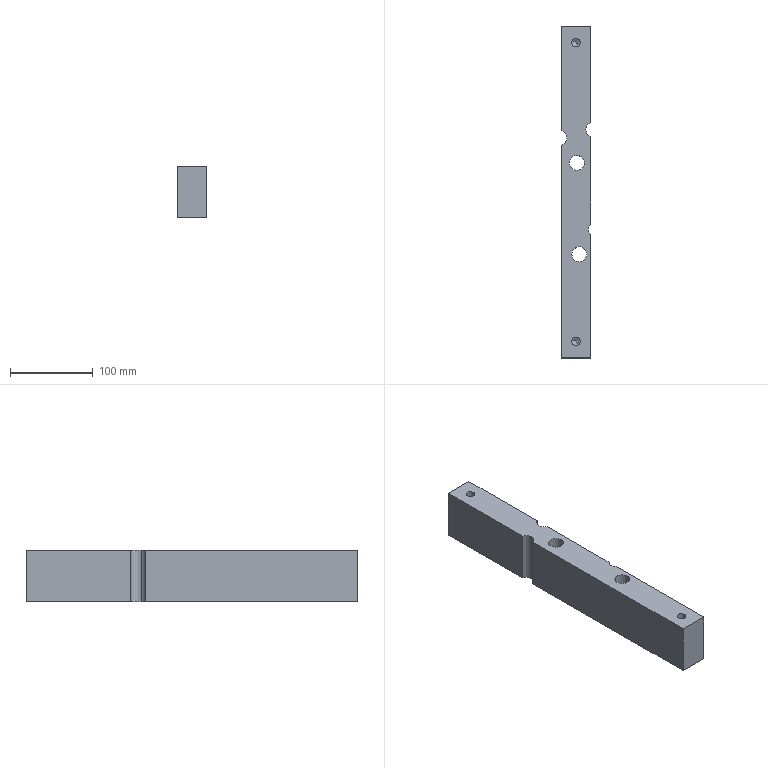Part | CATIA | 1 solid | 39 faces | box 35 x 400 x 61.7 mm | volume 807204 mm3 | cylinder 20 | cone 10 | plane 9 | commonest cylinder face diameters 10.2 x10 18 x10
STEP:
#1=CARTESIAN_POINT('',(-17.5,-200.,-275.));
#2=VERTEX_POINT('',#1);
#3=CARTESIAN_POINT('',(17.5,-200.,-275.));
#4=VERTEX_POINT('',#3);
#5=CARTESIAN_POINT('',(0.,-200.,-275.));
#6=DIRECTION('',(-1.,0.,0.));
#7=VECTOR('',#6,1.);
#8=LINE('',#5,#7);
#9=EDGE_CURVE('',#2,#4,#8,.F.);
#10=ORIENTED_EDGE('',*,*,#9,.T.);
#11=CARTESIAN_POINT('',(17.5,-200.,-213.3));
#12=VERTEX_POINT('',#11);
#13=CARTESIAN_POINT('',(17.5,-200.,-244.15));
#14=DIRECTION('',(0.,0.,-1.));
#15=VECTOR('',#14,1.);
#16=LINE('',#13,#15);
#17=EDGE_CURVE('',#12,#4,#16,.T.);
#18=ORIENTED_EDGE('',*,*,#17,.F.);
#19=CARTESIAN_POINT('',(-17.5,-200.,-213.3));
#20=VERTEX_POINT('',#19);
#21=CARTESIAN_POINT('',(0.,-200.,-213.3));
#22=DIRECTION('',(-1.,0.,0.));
#23=VECTOR('',#22,1.);
#24=LINE('',#21,#23);
#25=EDGE_CURVE('',#20,#12,#24,.F.);
#26=ORIENTED_EDGE('',*,*,#25,.F.);
#27=CARTESIAN_POINT('',(-17.5,-200.,-244.15));
#28=DIRECTION('',(0.,0.,-1.));
#29=VECTOR('',#28,1.);
#30=LINE('',#27,#29);
#31=EDGE_CURVE('',#20,#2,#30,.T.);
#32=ORIENTED_EDGE('',*,*,#31,.T.);
#33=EDGE_LOOP('',(#10,#18,#26,#32));
#34=FACE_OUTER_BOUND('',#33,.T.);
#35=CARTESIAN_POINT('',(17.5,-200.,0.));
#36=DIRECTION('',(0.,-1.,0.));
#37=DIRECTION('',(-1.,0.,0.));
#38=AXIS2_PLACEMENT_3D('',#35,#36,#37);
#39=PLANE('',#38);
#40=ADVANCED_FACE('',(#34),#39,.T.);
#41=CARTESIAN_POINT('',(17.5,200.,-275.));
#42=VERTEX_POINT('',#41);
#43=CARTESIAN_POINT('',(-17.5,200.,-275.));
#44=VERTEX_POINT('',#43);
#45=CARTESIAN_POINT('',(0.,200.,-275.));
#46=DIRECTION('',(1.,0.,0.));
#47=VECTOR('',#46,1.);
#48=LINE('',#45,#47);
#49=EDGE_CURVE('',#42,#44,#48,.F.);
#50=ORIENTED_EDGE('',*,*,#49,.T.);
#51=CARTESIAN_POINT('',(-17.5,200.,-213.3));
#52=VERTEX_POINT('',#51);
#53=CARTESIAN_POINT('',(-17.5,200.,-244.15));
#54=DIRECTION('',(0.,0.,-1.));
#55=VECTOR('',#54,1.);
#56=LINE('',#53,#55);
#57=EDGE_CURVE('',#52,#44,#56,.T.);
#58=ORIENTED_EDGE('',*,*,#57,.F.);
#59=CARTESIAN_POINT('',(17.5,200.,-213.3));
#60=VERTEX_POINT('',#59);
#61=CARTESIAN_POINT('',(0.,200.,-213.3));
#62=DIRECTION('',(1.,0.,0.));
#63=VECTOR('',#62,1.);
#64=LINE('',#61,#63);
#65=EDGE_CURVE('',#60,#52,#64,.F.);
#66=ORIENTED_EDGE('',*,*,#65,.F.);
#67=CARTESIAN_POINT('',(17.5,200.,-244.15));
#68=DIRECTION('',(0.,0.,-1.));
#69=VECTOR('',#68,1.);
#70=LINE('',#67,#69);
#71=EDGE_CURVE('',#60,#42,#70,.T.);
#72=ORIENTED_EDGE('',*,*,#71,.T.);
#73=EDGE_LOOP('',(#50,#58,#66,#72));
#74=FACE_OUTER_BOUND('',#73,.T.);
#75=CARTESIAN_POINT('',(-17.5,200.,0.));
#76=DIRECTION('',(0.,1.,0.));
#77=DIRECTION('',(1.,0.,0.));
#78=AXIS2_PLACEMENT_3D('',#75,#76,#77);
#79=PLANE('',#78);
#80=ADVANCED_FACE('',(#74),#79,.T.);
#81=CARTESIAN_POINT('',(17.5,-38.775,-213.3));
#82=VERTEX_POINT('',#81);
#83=CARTESIAN_POINT('',(17.5,-38.775,-275.));
#84=VERTEX_POINT('',#83);
#85=CARTESIAN_POINT('',(17.5,-38.775,-244.15));
#86=DIRECTION('',(0.,0.,-1.));
#87=VECTOR('',#86,1.);
#88=LINE('',#85,#87);
#89=EDGE_CURVE('',#82,#84,#88,.T.);
#90=ORIENTED_EDGE('',*,*,#89,.T.);
#91=CARTESIAN_POINT('',(17.5,66.708,-275.));
#92=VERTEX_POINT('',#91);
#93=CARTESIAN_POINT('',(17.5,13.967,-275.));
#94=DIRECTION('',(0.,1.,0.));
#95=VECTOR('',#94,1.);
#96=LINE('',#93,#95);
#97=EDGE_CURVE('',#84,#92,#96,.T.);
#98=ORIENTED_EDGE('',*,*,#97,.T.);
#99=CARTESIAN_POINT('',(17.5,66.708,-213.3));
#100=VERTEX_POINT('',#99);
#101=CARTESIAN_POINT('',(17.5,66.708,-244.15));
#102=DIRECTION('',(0.,0.,-1.));
#103=VECTOR('',#102,1.);
#104=LINE('',#101,#103);
#105=EDGE_CURVE('',#100,#92,#104,.T.);
#106=ORIENTED_EDGE('',*,*,#105,.F.);
#107=CARTESIAN_POINT('',(17.5,13.967,-213.3));
#108=DIRECTION('',(0.,1.,0.));
#109=VECTOR('',#108,1.);
#110=LINE('',#107,#109);
#111=EDGE_CURVE('',#82,#100,#110,.T.);
#112=ORIENTED_EDGE('',*,*,#111,.F.);
#113=EDGE_LOOP('',(#90,#98,#106,#112));
#114=FACE_OUTER_BOUND('',#113,.T.);
#115=CARTESIAN_POINT('',(17.5,-200.,0.));
#116=DIRECTION('',(-1.,0.,0.));
#117=DIRECTION('',(0.,1.,0.));
#118=AXIS2_PLACEMENT_3D('',#115,#116,#117);
#119=PLANE('',#118);
#120=ADVANCED_FACE('',(#114),#119,.F.);
#121=CARTESIAN_POINT('',(17.5,-51.225,-213.3));
#122=VERTEX_POINT('',#121);
#123=CARTESIAN_POINT('',(17.5,-51.225,-275.));
#124=VERTEX_POINT('',#123);
#125=CARTESIAN_POINT('',(17.5,-51.225,-244.15));
#126=DIRECTION('',(0.,0.,-1.));
#127=VECTOR('',#126,1.);
#128=LINE('',#125,#127);
#129=EDGE_CURVE('',#122,#124,#128,.T.);
#130=ORIENTED_EDGE('',*,*,#129,.F.);
#131=CARTESIAN_POINT('',(17.5,-125.612,-213.3));
#132=DIRECTION('',(0.,1.,0.));
#133=VECTOR('',#132,1.);
#134=LINE('',#131,#133);
#135=EDGE_CURVE('',#12,#122,#134,.T.);
#136=ORIENTED_EDGE('',*,*,#135,.F.);
#137=ORIENTED_EDGE('',*,*,#17,.T.);
#138=CARTESIAN_POINT('',(17.5,-125.612,-275.));
#139=DIRECTION('',(0.,1.,0.));
#140=VECTOR('',#139,1.);
#141=LINE('',#138,#140);
#142=EDGE_CURVE('',#4,#124,#141,.T.);
#143=ORIENTED_EDGE('',*,*,#142,.T.);
#144=EDGE_LOOP('',(#130,#136,#137,#143));
#145=FACE_OUTER_BOUND('',#144,.T.);
#146=ADVANCED_FACE('',(#145),#119,.F.);
#147=CARTESIAN_POINT('',(17.5,83.292,-213.3));
#148=VERTEX_POINT('',#147);
#149=CARTESIAN_POINT('',(17.5,83.292,-275.));
#150=VERTEX_POINT('',#149);
#151=CARTESIAN_POINT('',(17.5,83.292,-244.15));
#152=DIRECTION('',(0.,0.,-1.));
#153=VECTOR('',#152,1.);
#154=LINE('',#151,#153);
#155=EDGE_CURVE('',#148,#150,#154,.T.);
#156=ORIENTED_EDGE('',*,*,#155,.T.);
#157=CARTESIAN_POINT('',(17.5,141.646,-275.));
#158=DIRECTION('',(0.,1.,0.));
#159=VECTOR('',#158,1.);
#160=LINE('',#157,#159);
#161=EDGE_CURVE('',#150,#42,#160,.T.);
#162=ORIENTED_EDGE('',*,*,#161,.T.);
#163=ORIENTED_EDGE('',*,*,#71,.F.);
#164=CARTESIAN_POINT('',(17.5,141.646,-213.3));
#165=DIRECTION('',(0.,1.,0.));
#166=VECTOR('',#165,1.);
#167=LINE('',#164,#166);
#168=EDGE_CURVE('',#148,#60,#167,.T.);
#169=ORIENTED_EDGE('',*,*,#168,.F.);
#170=EDGE_LOOP('',(#156,#162,#163,#169));
#171=FACE_OUTER_BOUND('',#170,.T.);
#172=ADVANCED_FACE('',(#171),#119,.F.);
#173=CARTESIAN_POINT('',(-17.5,56.354,-213.3));
#174=VERTEX_POINT('',#173);
#175=CARTESIAN_POINT('',(-17.5,56.354,-275.));
#176=VERTEX_POINT('',#175);
#177=CARTESIAN_POINT('',(-17.5,56.354,-244.15));
#178=DIRECTION('',(0.,0.,-1.));
#179=VECTOR('',#178,1.);
#180=LINE('',#177,#179);
#181=EDGE_CURVE('',#174,#176,#180,.T.);
#182=ORIENTED_EDGE('',*,*,#181,.T.);
#183=CARTESIAN_POINT('',(-17.5,-71.823,-275.));
#184=DIRECTION('',(0.,-1.,0.));
#185=VECTOR('',#184,1.);
#186=LINE('',#183,#185);
#187=EDGE_CURVE('',#176,#2,#186,.T.);
#188=ORIENTED_EDGE('',*,*,#187,.T.);
#189=ORIENTED_EDGE('',*,*,#31,.F.);
#190=CARTESIAN_POINT('',(-17.5,-71.823,-213.3));
#191=DIRECTION('',(0.,-1.,0.));
#192=VECTOR('',#191,1.);
#193=LINE('',#190,#192);
#194=EDGE_CURVE('',#174,#20,#193,.T.);
#195=ORIENTED_EDGE('',*,*,#194,.F.);
#196=EDGE_LOOP('',(#182,#188,#189,#195));
#197=FACE_OUTER_BOUND('',#196,.T.);
#198=CARTESIAN_POINT('',(-17.5,200.,0.));
#199=DIRECTION('',(1.,0.,0.));
#200=DIRECTION('',(0.,-1.,0.));
#201=AXIS2_PLACEMENT_3D('',#198,#199,#200);
#202=PLANE('',#201);
#203=ADVANCED_FACE('',(#197),#202,.F.);
#204=CARTESIAN_POINT('',(-17.5,73.646,-213.3));
#205=VERTEX_POINT('',#204);
#206=CARTESIAN_POINT('',(-17.5,73.646,-275.));
#207=VERTEX_POINT('',#206);
#208=CARTESIAN_POINT('',(-17.5,73.646,-244.15));
#209=DIRECTION('',(0.,0.,-1.));
#210=VECTOR('',#209,1.);
#211=LINE('',#208,#210);
#212=EDGE_CURVE('',#205,#207,#211,.T.);
#213=ORIENTED_EDGE('',*,*,#212,.F.);
#214=CARTESIAN_POINT('',(-17.5,136.823,-213.3));
#215=DIRECTION('',(0.,-1.,0.));
#216=VECTOR('',#215,1.);
#217=LINE('',#214,#216);
#218=EDGE_CURVE('',#52,#205,#217,.T.);
#219=ORIENTED_EDGE('',*,*,#218,.F.);
#220=ORIENTED_EDGE('',*,*,#57,.T.);
#221=CARTESIAN_POINT('',(-17.5,136.823,-275.));
#222=DIRECTION('',(0.,-1.,0.));
#223=VECTOR('',#222,1.);
#224=LINE('',#221,#223);
#225=EDGE_CURVE('',#44,#207,#224,.T.);
#226=ORIENTED_EDGE('',*,*,#225,.T.);
#227=EDGE_LOOP('',(#213,#219,#220,#226));
#228=FACE_OUTER_BOUND('',#227,.T.);
#229=ADVANCED_FACE('',(#228),#202,.F.);
#230=CARTESIAN_POINT('',(11.898,-79.315,-275.));
#231=VERTEX_POINT('',#230);
#232=CARTESIAN_POINT('',(11.898,-79.315,-213.3));
#233=VERTEX_POINT('',#232);
#234=CARTESIAN_POINT('',(11.898,-79.315,-253.1));
#235=DIRECTION('',(0.,0.,-1.));
#236=VECTOR('',#235,1.);
#237=LINE('',#234,#236);
#238=EDGE_CURVE('',#231,#233,#237,.F.);
#239=ORIENTED_EDGE('',*,*,#238,.T.);
#240=CARTESIAN_POINT('',(-3.898,-70.685,-213.3));
#241=VERTEX_POINT('',#240);
#242=CARTESIAN_POINT('',(4.,-75.,-213.3));
#243=DIRECTION('',(0.,0.,-1.));
#244=AXIS2_PLACEMENT_3D('',#242,#243,$);
#245=CIRCLE('',#244,9.);
#246=EDGE_CURVE('',#233,#241,#245,.F.);
#247=ORIENTED_EDGE('',*,*,#246,.T.);
#248=CARTESIAN_POINT('',(-3.898,-70.685,-275.));
#249=VERTEX_POINT('',#248);
#250=CARTESIAN_POINT('',(-3.898,-70.685,-253.1));
#251=DIRECTION('',(0.,0.,-1.));
#252=VECTOR('',#251,1.);
#253=LINE('',#250,#252);
#254=EDGE_CURVE('',#249,#241,#253,.F.);
#255=ORIENTED_EDGE('',*,*,#254,.F.);
#256=CARTESIAN_POINT('',(4.,-75.,-275.));
#257=DIRECTION('',(0.,0.,-1.));
#258=AXIS2_PLACEMENT_3D('',#256,#257,$);
#259=CIRCLE('',#258,9.);
#260=EDGE_CURVE('',#231,#249,#259,.F.);
#261=ORIENTED_EDGE('',*,*,#260,.F.);
#262=EDGE_LOOP('',(#239,#247,#255,#261));
#263=FACE_OUTER_BOUND('',#262,.T.);
#264=CARTESIAN_POINT('',(4.,-75.,-178.4));
#265=DIRECTION('',(0.,0.,-1.));
#266=DIRECTION('',(-0.8776,0.4794,0.));
#267=AXIS2_PLACEMENT_3D('',#264,#265,#266);
#268=CYLINDRICAL_SURFACE('',#267,9.);
#269=ADVANCED_FACE('',(#263),#268,.F.);
#270=ORIENTED_EDGE('',*,*,#254,.T.);
#271=CARTESIAN_POINT('',(4.,-75.,-213.3));
#272=DIRECTION('',(0.,0.,-1.));
#273=AXIS2_PLACEMENT_3D('',#271,#272,$);
#274=CIRCLE('',#273,9.);
#275=EDGE_CURVE('',#241,#233,#274,.F.);
#276=ORIENTED_EDGE('',*,*,#275,.T.);
#277=ORIENTED_EDGE('',*,*,#238,.F.);
#278=CARTESIAN_POINT('',(4.,-75.,-275.));
#279=DIRECTION('',(0.,0.,-1.));
#280=AXIS2_PLACEMENT_3D('',#278,#279,$);
#281=CIRCLE('',#280,9.);
#282=EDGE_CURVE('',#249,#231,#281,.F.);
#283=ORIENTED_EDGE('',*,*,#282,.F.);
#284=EDGE_LOOP('',(#270,#276,#277,#283));
#285=FACE_OUTER_BOUND('',#284,.T.);
#286=ADVANCED_FACE('',(#285),#268,.F.);
#287=CARTESIAN_POINT('',(13.102,79.315,-275.));
#288=VERTEX_POINT('',#287);
#289=CARTESIAN_POINT('',(21.,75.,-275.));
#290=DIRECTION('',(0.,0.,-1.));
#291=AXIS2_PLACEMENT_3D('',#289,#290,$);
#292=CIRCLE('',#291,9.);
#293=EDGE_CURVE('',#150,#288,#292,.F.);
#294=ORIENTED_EDGE('',*,*,#293,.F.);
#295=ORIENTED_EDGE('',*,*,#155,.F.);
#296=CARTESIAN_POINT('',(13.102,79.315,-213.3));
#297=VERTEX_POINT('',#296);
#298=CARTESIAN_POINT('',(21.,75.,-213.3));
#299=DIRECTION('',(0.,0.,-1.));
#300=AXIS2_PLACEMENT_3D('',#298,#299,$);
#301=CIRCLE('',#300,9.);
#302=EDGE_CURVE('',#148,#297,#301,.F.);
#303=ORIENTED_EDGE('',*,*,#302,.T.);
#304=CARTESIAN_POINT('',(13.102,79.315,-253.1));
#305=DIRECTION('',(0.,0.,-1.));
#306=VECTOR('',#305,1.);
#307=LINE('',#304,#306);
#308=EDGE_CURVE('',#288,#297,#307,.F.);
#309=ORIENTED_EDGE('',*,*,#308,.F.);
#310=EDGE_LOOP('',(#294,#295,#303,#309));
#311=FACE_OUTER_BOUND('',#310,.T.);
#312=CARTESIAN_POINT('',(21.,75.,-178.4));
#313=DIRECTION('',(0.,0.,-1.));
#314=DIRECTION('',(-0.8776,0.4794,0.));
#315=AXIS2_PLACEMENT_3D('',#312,#313,#314);
#316=CYLINDRICAL_SURFACE('',#315,9.);
#317=ADVANCED_FACE('',(#311),#316,.F.);
#318=CARTESIAN_POINT('',(21.,75.,-213.3));
#319=DIRECTION('',(0.,0.,-1.));
#320=AXIS2_PLACEMENT_3D('',#318,#319,$);
#321=CIRCLE('',#320,9.);
#322=EDGE_CURVE('',#297,#100,#321,.F.);
#323=ORIENTED_EDGE('',*,*,#322,.T.);
#324=ORIENTED_EDGE('',*,*,#105,.T.);
#325=CARTESIAN_POINT('',(21.,75.,-275.));
#326=DIRECTION('',(0.,0.,-1.));
#327=AXIS2_PLACEMENT_3D('',#325,#326,$);
#328=CIRCLE('',#327,9.);
#329=EDGE_CURVE('',#288,#92,#328,.F.);
#330=ORIENTED_EDGE('',*,*,#329,.F.);
#331=ORIENTED_EDGE('',*,*,#308,.T.);
#332=EDGE_LOOP('',(#323,#324,#330,#331));
#333=FACE_OUTER_BOUND('',#332,.T.);
#334=ADVANCED_FACE('',(#333),#316,.F.);
#335=CARTESIAN_POINT('',(16.102,-40.685,-275.));
#336=VERTEX_POINT('',#335);
#337=CARTESIAN_POINT('',(24.,-45.,-275.));
#338=DIRECTION('',(0.,0.,-1.));
#339=AXIS2_PLACEMENT_3D('',#337,#338,$);
#340=CIRCLE('',#339,9.);
#341=EDGE_CURVE('',#84,#336,#340,.F.);
#342=ORIENTED_EDGE('',*,*,#341,.F.);
#343=ORIENTED_EDGE('',*,*,#89,.F.);
#344=CARTESIAN_POINT('',(16.102,-40.685,-213.3));
#345=VERTEX_POINT('',#344);
#346=CARTESIAN_POINT('',(24.,-45.,-213.3));
#347=DIRECTION('',(0.,0.,-1.));
#348=AXIS2_PLACEMENT_3D('',#346,#347,$);
#349=CIRCLE('',#348,9.);
#350=EDGE_CURVE('',#82,#345,#349,.F.);
#351=ORIENTED_EDGE('',*,*,#350,.T.);
#352=CARTESIAN_POINT('',(16.102,-40.685,-253.1));
#353=DIRECTION('',(0.,0.,-1.));
#354=VECTOR('',#353,1.);
#355=LINE('',#352,#354);
#356=EDGE_CURVE('',#336,#345,#355,.F.);
#357=ORIENTED_EDGE('',*,*,#356,.F.);
#358=EDGE_LOOP('',(#342,#343,#351,#357));
#359=FACE_OUTER_BOUND('',#358,.T.);
#360=CARTESIAN_POINT('',(24.,-45.,-178.4));
#361=DIRECTION('',(0.,0.,-1.));
#362=DIRECTION('',(-0.8776,0.4794,0.));
#363=AXIS2_PLACEMENT_3D('',#360,#361,#362);
#364=CYLINDRICAL_SURFACE('',#363,9.);
#365=ADVANCED_FACE('',(#359),#364,.F.);
#366=CARTESIAN_POINT('',(24.,-45.,-213.3));
#367=DIRECTION('',(0.,0.,-1.));
#368=AXIS2_PLACEMENT_3D('',#366,#367,$);
#369=CIRCLE('',#368,9.);
#370=EDGE_CURVE('',#345,#122,#369,.F.);
#371=ORIENTED_EDGE('',*,*,#370,.T.);
#372=ORIENTED_EDGE('',*,*,#129,.T.);
#373=CARTESIAN_POINT('',(24.,-45.,-275.));
#374=DIRECTION('',(0.,0.,-1.));
#375=AXIS2_PLACEMENT_3D('',#373,#374,$);
#376=CIRCLE('',#375,9.);
#377=EDGE_CURVE('',#336,#124,#376,.F.);
#378=ORIENTED_EDGE('',*,*,#377,.F.);
#379=ORIENTED_EDGE('',*,*,#356,.T.);
#380=EDGE_LOOP('',(#371,#372,#378,#379));
#381=FACE_OUTER_BOUND('',#380,.T.);
#382=ADVANCED_FACE('',(#381),#364,.F.);
#383=CARTESIAN_POINT('',(-12.102,60.685,-213.3));
#384=VERTEX_POINT('',#383);
#385=CARTESIAN_POINT('',(-20.,65.,-213.3));
#386=DIRECTION('',(0.,0.,-1.));
#387=AXIS2_PLACEMENT_3D('',#385,#386,$);
#388=CIRCLE('',#387,9.);
#389=EDGE_CURVE('',#384,#205,#388,.F.);
#390=ORIENTED_EDGE('',*,*,#389,.T.);
#391=ORIENTED_EDGE('',*,*,#212,.T.);
#392=CARTESIAN_POINT('',(-12.102,60.685,-275.));
#393=VERTEX_POINT('',#392);
#394=CARTESIAN_POINT('',(-20.,65.,-275.));
#395=DIRECTION('',(0.,0.,-1.));
#396=AXIS2_PLACEMENT_3D('',#394,#395,$);
#397=CIRCLE('',#396,9.);
#398=EDGE_CURVE('',#393,#207,#397,.F.);
#399=ORIENTED_EDGE('',*,*,#398,.F.);
#400=CARTESIAN_POINT('',(-12.102,60.685,-253.1));
#401=DIRECTION('',(0.,0.,-1.));
#402=VECTOR('',#401,1.);
#403=LINE('',#400,#402);
#404=EDGE_CURVE('',#393,#384,#403,.F.);
#405=ORIENTED_EDGE('',*,*,#404,.T.);
#406=EDGE_LOOP('',(#390,#391,#399,#405));
#407=FACE_OUTER_BOUND('',#406,.T.);
#408=CARTESIAN_POINT('',(-20.,65.,-178.4));
#409=DIRECTION('',(0.,0.,-1.));
#410=DIRECTION('',(-0.8776,0.4794,0.));
#411=AXIS2_PLACEMENT_3D('',#408,#409,#410);
#412=CYLINDRICAL_SURFACE('',#411,9.);
#413=ADVANCED_FACE('',(#407),#412,.F.);
#414=CARTESIAN_POINT('',(-20.,65.,-275.));
#415=DIRECTION('',(0.,0.,-1.));
#416=AXIS2_PLACEMENT_3D('',#414,#415,$);
#417=CIRCLE('',#416,9.);
#418=EDGE_CURVE('',#176,#393,#417,.F.);
#419=ORIENTED_EDGE('',*,*,#418,.F.);
#420=ORIENTED_EDGE('',*,*,#181,.F.);
#421=CARTESIAN_POINT('',(-20.,65.,-213.3));
#422=DIRECTION('',(0.,0.,-1.));
#423=AXIS2_PLACEMENT_3D('',#421,#422,$);
#424=CIRCLE('',#423,9.);
#425=EDGE_CURVE('',#174,#384,#424,.F.);
#426=ORIENTED_EDGE('',*,*,#425,.T.);
#427=ORIENTED_EDGE('',*,*,#404,.F.);
#428=EDGE_LOOP('',(#419,#420,#426,#427));
#429=FACE_OUTER_BOUND('',#428,.T.);
#430=ADVANCED_FACE('',(#429),#412,.F.);
#431=CARTESIAN_POINT('',(8.898,30.685,-275.));
#432=VERTEX_POINT('',#431);
#433=CARTESIAN_POINT('',(8.898,30.685,-213.3));
#434=VERTEX_POINT('',#433);
#435=CARTESIAN_POINT('',(8.898,30.685,-253.1));
#436=DIRECTION('',(0.,0.,-1.));
#437=VECTOR('',#436,1.);
#438=LINE('',#435,#437);
#439=EDGE_CURVE('',#432,#434,#438,.F.);
#440=ORIENTED_EDGE('',*,*,#439,.T.);
#441=CARTESIAN_POINT('',(-6.898,39.315,-213.3));
#442=VERTEX_POINT('',#441);
#443=CARTESIAN_POINT('',(1.,35.,-213.3));
#444=DIRECTION('',(0.,0.,-1.));
#445=AXIS2_PLACEMENT_3D('',#443,#444,$);
#446=CIRCLE('',#445,9.);
#447=EDGE_CURVE('',#434,#442,#446,.F.);
#448=ORIENTED_EDGE('',*,*,#447,.T.);
#449=CARTESIAN_POINT('',(-6.898,39.315,-275.));
#450=VERTEX_POINT('',#449);
#451=CARTESIAN_POINT('',(-6.898,39.315,-253.1));
#452=DIRECTION('',(0.,0.,-1.));
#453=VECTOR('',#452,1.);
#454=LINE('',#451,#453);
#455=EDGE_CURVE('',#450,#442,#454,.F.);
#456=ORIENTED_EDGE('',*,*,#455,.F.);
#457=CARTESIAN_POINT('',(1.,35.,-275.));
#458=DIRECTION('',(0.,0.,-1.));
#459=AXIS2_PLACEMENT_3D('',#457,#458,$);
#460=CIRCLE('',#459,9.);
#461=EDGE_CURVE('',#432,#450,#460,.F.);
#462=ORIENTED_EDGE('',*,*,#461,.F.);
#463=EDGE_LOOP('',(#440,#448,#456,#462));
#464=FACE_OUTER_BOUND('',#463,.T.);
#465=CARTESIAN_POINT('',(1.,35.,-178.4));
#466=DIRECTION('',(0.,0.,-1.));
#467=DIRECTION('',(-0.8776,0.4794,0.));
#468=AXIS2_PLACEMENT_3D('',#465,#466,#467);
#469=CYLINDRICAL_SURFACE('',#468,9.);
#470=ADVANCED_FACE('',(#464),#469,.F.);
#471=ORIENTED_EDGE('',*,*,#455,.T.);
#472=CARTESIAN_POINT('',(1.,35.,-213.3));
#473=DIRECTION('',(0.,0.,-1.));
#474=AXIS2_PLACEMENT_3D('',#472,#473,$);
#475=CIRCLE('',#474,9.);
#476=EDGE_CURVE('',#442,#434,#475,.F.);
#477=ORIENTED_EDGE('',*,*,#476,.T.);
#478=ORIENTED_EDGE('',*,*,#439,.F.);
#479=CARTESIAN_POINT('',(1.,35.,-275.));
#480=DIRECTION('',(0.,0.,-1.));
#481=AXIS2_PLACEMENT_3D('',#479,#480,$);
#482=CIRCLE('',#481,9.);
#483=EDGE_CURVE('',#450,#432,#482,.F.);
#484=ORIENTED_EDGE('',*,*,#483,.F.);
#485=EDGE_LOOP('',(#471,#477,#478,#484));
#486=FACE_OUTER_BOUND('',#485,.T.);
#487=ADVANCED_FACE('',(#486),#469,.F.);
#488=ORIENTED_EDGE('',*,*,#194,.T.);
#489=ORIENTED_EDGE('',*,*,#25,.T.);
#490=ORIENTED_EDGE('',*,*,#135,.T.);
#491=ORIENTED_EDGE('',*,*,#370,.F.);
#492=ORIENTED_EDGE('',*,*,#350,.F.);
#493=ORIENTED_EDGE('',*,*,#111,.T.);
#494=ORIENTED_EDGE('',*,*,#322,.F.);
#495=ORIENTED_EDGE('',*,*,#302,.F.);
#496=ORIENTED_EDGE('',*,*,#168,.T.);
#497=ORIENTED_EDGE('',*,*,#65,.T.);
#498=ORIENTED_EDGE('',*,*,#218,.T.);
#499=ORIENTED_EDGE('',*,*,#389,.F.);
#500=ORIENTED_EDGE('',*,*,#425,.F.);
#501=EDGE_LOOP('',(#488,#489,#490,#491,#492,#493,#494,#495,#496,#497,#498,#499,#500));
#502=FACE_OUTER_BOUND('',#501,.T.);
#503=ORIENTED_EDGE('',*,*,#476,.F.);
#504=ORIENTED_EDGE('',*,*,#447,.F.);
#505=EDGE_LOOP('',(#503,#504));
#506=FACE_BOUND('',#505,.T.);
#507=ORIENTED_EDGE('',*,*,#275,.F.);
#508=ORIENTED_EDGE('',*,*,#246,.F.);
#509=EDGE_LOOP('',(#507,#508));
#510=FACE_BOUND('',#509,.T.);
#511=CARTESIAN_POINT('',(4.476,-182.445,-213.3));
#512=VERTEX_POINT('',#511);
#513=CARTESIAN_POINT('',(-4.476,-177.555,-213.3));
#514=VERTEX_POINT('',#513);
#515=CARTESIAN_POINT('',(0.,-180.,-213.3));
#516=DIRECTION('',(0.,0.,1.));
#517=AXIS2_PLACEMENT_3D('',#515,#516,$);
#518=CIRCLE('',#517,5.1);
#519=EDGE_CURVE('',#512,#514,#518,.T.);
#520=ORIENTED_EDGE('',*,*,#519,.F.);
#521=CARTESIAN_POINT('',(0.,-180.,-213.3));
#522=DIRECTION('',(0.,0.,1.));
#523=AXIS2_PLACEMENT_3D('',#521,#522,$);
#524=CIRCLE('',#523,5.1);
#525=EDGE_CURVE('',#514,#512,#524,.T.);
#526=ORIENTED_EDGE('',*,*,#525,.F.);
#527=EDGE_LOOP('',(#520,#526));
#528=FACE_BOUND('',#527,.T.);
#529=CARTESIAN_POINT('',(4.476,177.555,-213.3));
#530=VERTEX_POINT('',#529);
#531=CARTESIAN_POINT('',(-4.476,182.445,-213.3));
#532=VERTEX_POINT('',#531);
#533=CARTESIAN_POINT('',(0.,180.,-213.3));
#534=DIRECTION('',(0.,0.,1.));
#535=AXIS2_PLACEMENT_3D('',#533,#534,$);
#536=CIRCLE('',#535,5.1);
#537=EDGE_CURVE('',#530,#532,#536,.T.);
#538=ORIENTED_EDGE('',*,*,#537,.F.);
#539=CARTESIAN_POINT('',(0.,180.,-213.3));
#540=DIRECTION('',(0.,0.,1.));
#541=AXIS2_PLACEMENT_3D('',#539,#540,$);
#542=CIRCLE('',#541,5.1);
#543=EDGE_CURVE('',#532,#530,#542,.T.);
#544=ORIENTED_EDGE('',*,*,#543,.F.);
#545=EDGE_LOOP('',(#538,#544));
#546=FACE_BOUND('',#545,.T.);
#547=CARTESIAN_POINT('',(0.,0.,-213.3));
#548=DIRECTION('',(0.,0.,1.));
#549=DIRECTION('',(1.,0.,0.));
#550=AXIS2_PLACEMENT_3D('',#547,#548,#549);
#551=PLANE('',#550);
#552=ADVANCED_FACE('',(#502,#506,#510,#528,#546),#551,.T.);
#553=ORIENTED_EDGE('',*,*,#418,.T.);
#554=ORIENTED_EDGE('',*,*,#398,.T.);
#555=ORIENTED_EDGE('',*,*,#225,.F.);
#556=ORIENTED_EDGE('',*,*,#49,.F.);
#557=ORIENTED_EDGE('',*,*,#161,.F.);
#558=ORIENTED_EDGE('',*,*,#293,.T.);
#559=ORIENTED_EDGE('',*,*,#329,.T.);
#560=ORIENTED_EDGE('',*,*,#97,.F.);
#561=ORIENTED_EDGE('',*,*,#341,.T.);
#562=ORIENTED_EDGE('',*,*,#377,.T.);
#563=ORIENTED_EDGE('',*,*,#142,.F.);
#564=ORIENTED_EDGE('',*,*,#9,.F.);
#565=ORIENTED_EDGE('',*,*,#187,.F.);
#566=EDGE_LOOP('',(#553,#554,#555,#556,#557,#558,#559,#560,#561,#562,#563,#564,#565));
#567=FACE_OUTER_BOUND('',#566,.T.);
#568=ORIENTED_EDGE('',*,*,#461,.T.);
#569=ORIENTED_EDGE('',*,*,#483,.T.);
#570=EDGE_LOOP('',(#568,#569));
#571=FACE_BOUND('',#570,.T.);
#572=ORIENTED_EDGE('',*,*,#260,.T.);
#573=ORIENTED_EDGE('',*,*,#282,.T.);
#574=EDGE_LOOP('',(#572,#573));
#575=FACE_BOUND('',#574,.T.);
#576=CARTESIAN_POINT('',(4.476,-162.555,-275.));
#577=VERTEX_POINT('',#576);
#578=CARTESIAN_POINT('',(-4.476,-167.445,-275.));
#579=VERTEX_POINT('',#578);
#580=CARTESIAN_POINT('',(0.,-165.,-275.));
#581=DIRECTION('',(0.,0.,1.));
#582=AXIS2_PLACEMENT_3D('',#580,#581,$);
#583=CIRCLE('',#582,5.1);
#584=EDGE_CURVE('',#577,#579,#583,.T.);
#585=ORIENTED_EDGE('',*,*,#584,.T.);
#586=CARTESIAN_POINT('',(0.,-165.,-275.));
#587=DIRECTION('',(0.,0.,1.));
#588=AXIS2_PLACEMENT_3D('',#586,#587,$);
#589=CIRCLE('',#588,5.1);
#590=EDGE_CURVE('',#579,#577,#589,.T.);
#591=ORIENTED_EDGE('',*,*,#590,.T.);
#592=EDGE_LOOP('',(#585,#591));
#593=FACE_BOUND('',#592,.T.);
#594=CARTESIAN_POINT('',(4.476,167.445,-275.));
#595=VERTEX_POINT('',#594);
#596=CARTESIAN_POINT('',(-4.476,162.555,-275.));
#597=VERTEX_POINT('',#596);
#598=CARTESIAN_POINT('',(0.,165.,-275.));
#599=DIRECTION('',(0.,0.,1.));
#600=AXIS2_PLACEMENT_3D('',#598,#599,$);
#601=CIRCLE('',#600,5.1);
#602=EDGE_CURVE('',#595,#597,#601,.T.);
#603=ORIENTED_EDGE('',*,*,#602,.T.);
#604=CARTESIAN_POINT('',(0.,165.,-275.));
#605=DIRECTION('',(0.,0.,1.));
#606=AXIS2_PLACEMENT_3D('',#604,#605,$);
#607=CIRCLE('',#606,5.1);
#608=EDGE_CURVE('',#597,#595,#607,.T.);
#609=ORIENTED_EDGE('',*,*,#608,.T.);
#610=EDGE_LOOP('',(#603,#609));
#611=FACE_BOUND('',#610,.T.);
#612=CARTESIAN_POINT('',(4.476,12.445,-275.));
#613=VERTEX_POINT('',#612);
#614=CARTESIAN_POINT('',(-4.476,7.555,-275.));
#615=VERTEX_POINT('',#614);
#616=CARTESIAN_POINT('',(0.,10.,-275.));
#617=DIRECTION('',(0.,0.,1.));
#618=AXIS2_PLACEMENT_3D('',#616,#617,$);
#619=CIRCLE('',#618,5.1);
#620=EDGE_CURVE('',#613,#615,#619,.T.);
#621=ORIENTED_EDGE('',*,*,#620,.T.);
#622=CARTESIAN_POINT('',(0.,10.,-275.));
#623=DIRECTION('',(0.,0.,1.));
#624=AXIS2_PLACEMENT_3D('',#622,#623,$);
#625=CIRCLE('',#624,5.1);
#626=EDGE_CURVE('',#615,#613,#625,.T.);
#627=ORIENTED_EDGE('',*,*,#626,.T.);
#628=EDGE_LOOP('',(#621,#627));
#629=FACE_BOUND('',#628,.T.);
#630=CARTESIAN_POINT('',(0.,0.,-275.));
#631=DIRECTION('',(0.,0.,1.));
#632=DIRECTION('',(1.,0.,0.));
#633=AXIS2_PLACEMENT_3D('',#630,#631,#632);
#634=PLANE('',#633);
#635=ADVANCED_FACE('',(#567,#571,#575,#593,#611,#629),#634,.F.);
#636=CARTESIAN_POINT('',(0.,10.,-237.056));
#637=VERTEX_POINT('',#636);
#638=CARTESIAN_POINT('',(-4.476,7.555,-240.));
#639=VERTEX_POINT('',#638);
#640=CARTESIAN_POINT('',(-2.238,8.777,-238.528));
#641=DIRECTION('',(-0.76,-0.4152,-0.5));
#642=VECTOR('',#641,1.);
#643=LINE('',#640,#642);
#644=EDGE_CURVE('',#637,#639,#643,.T.);
#645=ORIENTED_EDGE('',*,*,#644,.T.);
#646=CARTESIAN_POINT('',(4.476,12.445,-240.));
#647=VERTEX_POINT('',#646);
#648=CARTESIAN_POINT('',(0.,10.,-240.));
#649=DIRECTION('',(0.,0.,-1.));
#650=AXIS2_PLACEMENT_3D('',#648,#649,$);
#651=CIRCLE('',#650,5.1);
#652=EDGE_CURVE('',#647,#639,#651,.F.);
#653=ORIENTED_EDGE('',*,*,#652,.F.);
#654=CARTESIAN_POINT('',(2.238,11.223,-238.528));
#655=DIRECTION('',(0.76,0.4152,-0.5));
#656=VECTOR('',#655,1.);
#657=LINE('',#654,#656);
#658=EDGE_CURVE('',#637,#647,#657,.T.);
#659=ORIENTED_EDGE('',*,*,#658,.F.);
#660=EDGE_LOOP('',(#645,#653,#659));
#661=FACE_OUTER_BOUND('',#660,.T.);
#662=CARTESIAN_POINT('',(0.,10.,-237.056));
#663=DIRECTION('',(0.,0.,-1.));
#664=DIRECTION('',(0.8776,0.4794,0.));
#665=AXIS2_PLACEMENT_3D('',#662,#663,#664);
#666=CONICAL_SURFACE('',#665,0.,1.047);
#667=ADVANCED_FACE('',(#661),#666,.F.);
#668=ORIENTED_EDGE('',*,*,#658,.T.);
#669=CARTESIAN_POINT('',(0.,10.,-240.));
#670=DIRECTION('',(0.,0.,-1.));
#671=AXIS2_PLACEMENT_3D('',#669,#670,$);
#672=CIRCLE('',#671,5.1);
#673=EDGE_CURVE('',#639,#647,#672,.F.);
#674=ORIENTED_EDGE('',*,*,#673,.F.);
#675=ORIENTED_EDGE('',*,*,#644,.F.);
#676=EDGE_LOOP('',(#668,#674,#675));
#677=FACE_OUTER_BOUND('',#676,.T.);
#678=ADVANCED_FACE('',(#677),#666,.F.);
#679=ORIENTED_EDGE('',*,*,#620,.F.);
#680=CARTESIAN_POINT('',(4.476,12.445,-257.7));
#681=DIRECTION('',(0.,0.,1.));
#682=VECTOR('',#681,1.);
#683=LINE('',#680,#682);
#684=EDGE_CURVE('',#647,#613,#683,.F.);
#685=ORIENTED_EDGE('',*,*,#684,.F.);
#686=ORIENTED_EDGE('',*,*,#652,.T.);
#687=CARTESIAN_POINT('',(-4.476,7.555,-257.7));
#688=DIRECTION('',(0.,0.,1.));
#689=VECTOR('',#688,1.);
#690=LINE('',#687,#689);
#691=EDGE_CURVE('',#639,#615,#690,.F.);
#692=ORIENTED_EDGE('',*,*,#691,.T.);
#693=EDGE_LOOP('',(#679,#685,#686,#692));
#694=FACE_OUTER_BOUND('',#693,.T.);
#695=CARTESIAN_POINT('',(0.,10.,-274.9));
#696=DIRECTION('',(0.,0.,1.));
#697=DIRECTION('',(0.8776,0.4794,0.));
#698=AXIS2_PLACEMENT_3D('',#695,#696,#697);
#699=CYLINDRICAL_SURFACE('',#698,5.1);
#700=ADVANCED_FACE('',(#694),#699,.F.);
#701=ORIENTED_EDGE('',*,*,#626,.F.);
#702=ORIENTED_EDGE('',*,*,#691,.F.);
#703=ORIENTED_EDGE('',*,*,#673,.T.);
#704=ORIENTED_EDGE('',*,*,#684,.T.);
#705=EDGE_LOOP('',(#701,#702,#703,#704));
#706=FACE_OUTER_BOUND('',#705,.T.);
#707=ADVANCED_FACE('',(#706),#699,.F.);
#708=CARTESIAN_POINT('',(0.,180.,-251.244));
#709=VERTEX_POINT('',#708);
#710=CARTESIAN_POINT('',(-4.476,182.445,-248.3));
#711=VERTEX_POINT('',#710);
#712=CARTESIAN_POINT('',(-2.238,181.223,-249.772));
#713=DIRECTION('',(-0.76,0.4152,0.5));
#714=VECTOR('',#713,1.);
#715=LINE('',#712,#714);
#716=EDGE_CURVE('',#709,#711,#715,.T.);
#717=ORIENTED_EDGE('',*,*,#716,.T.);
#718=CARTESIAN_POINT('',(4.476,177.555,-248.3));
#719=VERTEX_POINT('',#718);
#720=CARTESIAN_POINT('',(0.,180.,-248.3));
#721=DIRECTION('',(0.,0.,1.));
#722=AXIS2_PLACEMENT_3D('',#720,#721,$);
#723=CIRCLE('',#722,5.1);
#724=EDGE_CURVE('',#719,#711,#723,.F.);
#725=ORIENTED_EDGE('',*,*,#724,.F.);
#726=CARTESIAN_POINT('',(2.238,178.777,-249.772));
#727=DIRECTION('',(0.76,-0.4152,0.5));
#728=VECTOR('',#727,1.);
#729=LINE('',#726,#728);
#730=EDGE_CURVE('',#709,#719,#729,.T.);
#731=ORIENTED_EDGE('',*,*,#730,.F.);
#732=EDGE_LOOP('',(#717,#725,#731));
#733=FACE_OUTER_BOUND('',#732,.T.);
#734=CARTESIAN_POINT('',(0.,180.,-251.244));
#735=DIRECTION('',(0.,0.,1.));
#736=DIRECTION('',(0.8776,-0.4794,0.));
#737=AXIS2_PLACEMENT_3D('',#734,#735,#736);
#738=CONICAL_SURFACE('',#737,0.,1.047);
#739=ADVANCED_FACE('',(#733),#738,.F.);
#740=ORIENTED_EDGE('',*,*,#730,.T.);
#741=CARTESIAN_POINT('',(0.,180.,-248.3));
#742=DIRECTION('',(0.,0.,1.));
#743=AXIS2_PLACEMENT_3D('',#741,#742,$);
#744=CIRCLE('',#743,5.1);
#745=EDGE_CURVE('',#711,#719,#744,.F.);
#746=ORIENTED_EDGE('',*,*,#745,.F.);
#747=ORIENTED_EDGE('',*,*,#716,.F.);
#748=EDGE_LOOP('',(#740,#746,#747));
#749=FACE_OUTER_BOUND('',#748,.T.);
#750=ADVANCED_FACE('',(#749),#738,.F.);
#751=ORIENTED_EDGE('',*,*,#543,.T.);
#752=CARTESIAN_POINT('',(4.476,177.555,-230.6));
#753=DIRECTION('',(0.,0.,-1.));
#754=VECTOR('',#753,1.);
#755=LINE('',#752,#754);
#756=EDGE_CURVE('',#719,#530,#755,.F.);
#757=ORIENTED_EDGE('',*,*,#756,.F.);
#758=ORIENTED_EDGE('',*,*,#724,.T.);
#759=CARTESIAN_POINT('',(-4.476,182.445,-230.6));
#760=DIRECTION('',(0.,0.,-1.));
#761=VECTOR('',#760,1.);
#762=LINE('',#759,#761);
#763=EDGE_CURVE('',#711,#532,#762,.F.);
#764=ORIENTED_EDGE('',*,*,#763,.T.);
#765=EDGE_LOOP('',(#751,#757,#758,#764));
#766=FACE_OUTER_BOUND('',#765,.T.);
#767=CARTESIAN_POINT('',(0.,180.,-213.4));
#768=DIRECTION('',(0.,0.,-1.));
#769=DIRECTION('',(0.8776,-0.4794,0.));
#770=AXIS2_PLACEMENT_3D('',#767,#768,#769);
#771=CYLINDRICAL_SURFACE('',#770,5.1);
#772=ADVANCED_FACE('',(#766),#771,.F.);
#773=ORIENTED_EDGE('',*,*,#537,.T.);
#774=ORIENTED_EDGE('',*,*,#763,.F.);
#775=ORIENTED_EDGE('',*,*,#745,.T.);
#776=ORIENTED_EDGE('',*,*,#756,.T.);
#777=EDGE_LOOP('',(#773,#774,#775,#776));
#778=FACE_OUTER_BOUND('',#777,.T.);
#779=ADVANCED_FACE('',(#778),#771,.F.);
#780=CARTESIAN_POINT('',(0.,165.,-237.056));
#781=VERTEX_POINT('',#780);
#782=CARTESIAN_POINT('',(-4.476,162.555,-240.));
#783=VERTEX_POINT('',#782);
#784=CARTESIAN_POINT('',(-2.238,163.777,-238.528));
#785=DIRECTION('',(-0.76,-0.4152,-0.5));
#786=VECTOR('',#785,1.);
#787=LINE('',#784,#786);
#788=EDGE_CURVE('',#781,#783,#787,.T.);
#789=ORIENTED_EDGE('',*,*,#788,.T.);
#790=CARTESIAN_POINT('',(4.476,167.445,-240.));
#791=VERTEX_POINT('',#790);
#792=CARTESIAN_POINT('',(0.,165.,-240.));
#793=DIRECTION('',(0.,0.,-1.));
#794=AXIS2_PLACEMENT_3D('',#792,#793,$);
#795=CIRCLE('',#794,5.1);
#796=EDGE_CURVE('',#791,#783,#795,.F.);
#797=ORIENTED_EDGE('',*,*,#796,.F.);
#798=CARTESIAN_POINT('',(2.238,166.223,-238.528));
#799=DIRECTION('',(0.76,0.4152,-0.5));
#800=VECTOR('',#799,1.);
#801=LINE('',#798,#800);
#802=EDGE_CURVE('',#781,#791,#801,.T.);
#803=ORIENTED_EDGE('',*,*,#802,.F.);
#804=EDGE_LOOP('',(#789,#797,#803));
#805=FACE_OUTER_BOUND('',#804,.T.);
#806=CARTESIAN_POINT('',(0.,165.,-237.056));
#807=DIRECTION('',(0.,0.,-1.));
#808=DIRECTION('',(0.8776,0.4794,0.));
#809=AXIS2_PLACEMENT_3D('',#806,#807,#808);
#810=CONICAL_SURFACE('',#809,0.,1.047);
#811=ADVANCED_FACE('',(#805),#810,.F.);
#812=ORIENTED_EDGE('',*,*,#802,.T.);
#813=CARTESIAN_POINT('',(0.,165.,-240.));
#814=DIRECTION('',(0.,0.,-1.));
#815=AXIS2_PLACEMENT_3D('',#813,#814,$);
#816=CIRCLE('',#815,5.1);
#817=EDGE_CURVE('',#783,#791,#816,.F.);
#818=ORIENTED_EDGE('',*,*,#817,.F.);
#819=ORIENTED_EDGE('',*,*,#788,.F.);
#820=EDGE_LOOP('',(#812,#818,#819));
#821=FACE_OUTER_BOUND('',#820,.T.);
#822=ADVANCED_FACE('',(#821),#810,.F.);
#823=ORIENTED_EDGE('',*,*,#602,.F.);
#824=CARTESIAN_POINT('',(4.476,167.445,-257.7));
#825=DIRECTION('',(0.,0.,1.));
#826=VECTOR('',#825,1.);
#827=LINE('',#824,#826);
#828=EDGE_CURVE('',#791,#595,#827,.F.);
#829=ORIENTED_EDGE('',*,*,#828,.F.);
#830=ORIENTED_EDGE('',*,*,#796,.T.);
#831=CARTESIAN_POINT('',(-4.476,162.555,-257.7));
#832=DIRECTION('',(0.,0.,1.));
#833=VECTOR('',#832,1.);
#834=LINE('',#831,#833);
#835=EDGE_CURVE('',#783,#597,#834,.F.);
#836=ORIENTED_EDGE('',*,*,#835,.T.);
#837=EDGE_LOOP('',(#823,#829,#830,#836));
#838=FACE_OUTER_BOUND('',#837,.T.);
#839=CARTESIAN_POINT('',(0.,165.,-274.9));
#840=DIRECTION('',(0.,0.,1.));
#841=DIRECTION('',(0.8776,0.4794,0.));
#842=AXIS2_PLACEMENT_3D('',#839,#840,#841);
#843=CYLINDRICAL_SURFACE('',#842,5.1);
#844=ADVANCED_FACE('',(#838),#843,.F.);
#845=ORIENTED_EDGE('',*,*,#608,.F.);
#846=ORIENTED_EDGE('',*,*,#835,.F.);
#847=ORIENTED_EDGE('',*,*,#817,.T.);
#848=ORIENTED_EDGE('',*,*,#828,.T.);
#849=EDGE_LOOP('',(#845,#846,#847,#848));
#850=FACE_OUTER_BOUND('',#849,.T.);
#851=ADVANCED_FACE('',(#850),#843,.F.);
#852=CARTESIAN_POINT('',(0.,-165.,-237.056));
#853=VERTEX_POINT('',#852);
#854=CARTESIAN_POINT('',(-4.476,-167.445,-240.));
#855=VERTEX_POINT('',#854);
#856=CARTESIAN_POINT('',(-2.238,-166.223,-238.528));
#857=DIRECTION('',(-0.76,-0.4152,-0.5));
#858=VECTOR('',#857,1.);
#859=LINE('',#856,#858);
#860=EDGE_CURVE('',#853,#855,#859,.T.);
#861=ORIENTED_EDGE('',*,*,#860,.T.);
#862=CARTESIAN_POINT('',(4.476,-162.555,-240.));
#863=VERTEX_POINT('',#862);
#864=CARTESIAN_POINT('',(0.,-165.,-240.));
#865=DIRECTION('',(0.,0.,-1.));
#866=AXIS2_PLACEMENT_3D('',#864,#865,$);
#867=CIRCLE('',#866,5.1);
#868=EDGE_CURVE('',#863,#855,#867,.F.);
#869=ORIENTED_EDGE('',*,*,#868,.F.);
#870=CARTESIAN_POINT('',(2.238,-163.777,-238.528));
#871=DIRECTION('',(0.76,0.4152,-0.5));
#872=VECTOR('',#871,1.);
#873=LINE('',#870,#872);
#874=EDGE_CURVE('',#853,#863,#873,.T.);
#875=ORIENTED_EDGE('',*,*,#874,.F.);
#876=EDGE_LOOP('',(#861,#869,#875));
#877=FACE_OUTER_BOUND('',#876,.T.);
#878=CARTESIAN_POINT('',(0.,-165.,-237.056));
#879=DIRECTION('',(0.,0.,-1.));
#880=DIRECTION('',(0.8776,0.4794,0.));
#881=AXIS2_PLACEMENT_3D('',#878,#879,#880);
#882=CONICAL_SURFACE('',#881,0.,1.047);
#883=ADVANCED_FACE('',(#877),#882,.F.);
#884=ORIENTED_EDGE('',*,*,#874,.T.);
#885=CARTESIAN_POINT('',(0.,-165.,-240.));
#886=DIRECTION('',(0.,0.,-1.));
#887=AXIS2_PLACEMENT_3D('',#885,#886,$);
#888=CIRCLE('',#887,5.1);
#889=EDGE_CURVE('',#855,#863,#888,.F.);
#890=ORIENTED_EDGE('',*,*,#889,.F.);
#891=ORIENTED_EDGE('',*,*,#860,.F.);
#892=EDGE_LOOP('',(#884,#890,#891));
#893=FACE_OUTER_BOUND('',#892,.T.);
#894=ADVANCED_FACE('',(#893),#882,.F.);
#895=ORIENTED_EDGE('',*,*,#584,.F.);
#896=CARTESIAN_POINT('',(4.476,-162.555,-257.7));
#897=DIRECTION('',(0.,0.,1.));
#898=VECTOR('',#897,1.);
#899=LINE('',#896,#898);
#900=EDGE_CURVE('',#863,#577,#899,.F.);
#901=ORIENTED_EDGE('',*,*,#900,.F.);
#902=ORIENTED_EDGE('',*,*,#868,.T.);
#903=CARTESIAN_POINT('',(-4.476,-167.445,-257.7));
#904=DIRECTION('',(0.,0.,1.));
#905=VECTOR('',#904,1.);
#906=LINE('',#903,#905);
#907=EDGE_CURVE('',#855,#579,#906,.F.);
#908=ORIENTED_EDGE('',*,*,#907,.T.);
#909=EDGE_LOOP('',(#895,#901,#902,#908));
#910=FACE_OUTER_BOUND('',#909,.T.);
#911=CARTESIAN_POINT('',(0.,-165.,-274.9));
#912=DIRECTION('',(0.,0.,1.));
#913=DIRECTION('',(0.8776,0.4794,0.));
#914=AXIS2_PLACEMENT_3D('',#911,#912,#913);
#915=CYLINDRICAL_SURFACE('',#914,5.1);
#916=ADVANCED_FACE('',(#910),#915,.F.);
#917=ORIENTED_EDGE('',*,*,#590,.F.);
#918=ORIENTED_EDGE('',*,*,#907,.F.);
#919=ORIENTED_EDGE('',*,*,#889,.T.);
#920=ORIENTED_EDGE('',*,*,#900,.T.);
#921=EDGE_LOOP('',(#917,#918,#919,#920));
#922=FACE_OUTER_BOUND('',#921,.T.);
#923=ADVANCED_FACE('',(#922),#915,.F.);
#924=CARTESIAN_POINT('',(0.,-180.,-251.244));
#925=VERTEX_POINT('',#924);
#926=CARTESIAN_POINT('',(-4.476,-177.555,-248.3));
#927=VERTEX_POINT('',#926);
#928=CARTESIAN_POINT('',(-2.238,-178.777,-249.772));
#929=DIRECTION('',(-0.76,0.4152,0.5));
#930=VECTOR('',#929,1.);
#931=LINE('',#928,#930);
#932=EDGE_CURVE('',#925,#927,#931,.T.);
#933=ORIENTED_EDGE('',*,*,#932,.T.);
#934=CARTESIAN_POINT('',(4.476,-182.445,-248.3));
#935=VERTEX_POINT('',#934);
#936=CARTESIAN_POINT('',(0.,-180.,-248.3));
#937=DIRECTION('',(0.,0.,1.));
#938=AXIS2_PLACEMENT_3D('',#936,#937,$);
#939=CIRCLE('',#938,5.1);
#940=EDGE_CURVE('',#935,#927,#939,.F.);
#941=ORIENTED_EDGE('',*,*,#940,.F.);
#942=CARTESIAN_POINT('',(2.238,-181.223,-249.772));
#943=DIRECTION('',(0.76,-0.4152,0.5));
#944=VECTOR('',#943,1.);
#945=LINE('',#942,#944);
#946=EDGE_CURVE('',#925,#935,#945,.T.);
#947=ORIENTED_EDGE('',*,*,#946,.F.);
#948=EDGE_LOOP('',(#933,#941,#947));
#949=FACE_OUTER_BOUND('',#948,.T.);
#950=CARTESIAN_POINT('',(0.,-180.,-251.244));
#951=DIRECTION('',(0.,0.,1.));
#952=DIRECTION('',(0.8776,-0.4794,0.));
#953=AXIS2_PLACEMENT_3D('',#950,#951,#952);
#954=CONICAL_SURFACE('',#953,0.,1.047);
#955=ADVANCED_FACE('',(#949),#954,.F.);
#956=ORIENTED_EDGE('',*,*,#946,.T.);
#957=CARTESIAN_POINT('',(0.,-180.,-248.3));
#958=DIRECTION('',(0.,0.,1.));
#959=AXIS2_PLACEMENT_3D('',#957,#958,$);
#960=CIRCLE('',#959,5.1);
#961=EDGE_CURVE('',#927,#935,#960,.F.);
#962=ORIENTED_EDGE('',*,*,#961,.F.);
#963=ORIENTED_EDGE('',*,*,#932,.F.);
#964=EDGE_LOOP('',(#956,#962,#963));
#965=FACE_OUTER_BOUND('',#964,.T.);
#966=ADVANCED_FACE('',(#965),#954,.F.);
#967=ORIENTED_EDGE('',*,*,#525,.T.);
#968=CARTESIAN_POINT('',(4.476,-182.445,-230.6));
#969=DIRECTION('',(0.,0.,-1.));
#970=VECTOR('',#969,1.);
#971=LINE('',#968,#970);
#972=EDGE_CURVE('',#935,#512,#971,.F.);
#973=ORIENTED_EDGE('',*,*,#972,.F.);
#974=ORIENTED_EDGE('',*,*,#940,.T.);
#975=CARTESIAN_POINT('',(-4.476,-177.555,-230.6));
#976=DIRECTION('',(0.,0.,-1.));
#977=VECTOR('',#976,1.);
#978=LINE('',#975,#977);
#979=EDGE_CURVE('',#927,#514,#978,.F.);
#980=ORIENTED_EDGE('',*,*,#979,.T.);
#981=EDGE_LOOP('',(#967,#973,#974,#980));
#982=FACE_OUTER_BOUND('',#981,.T.);
#983=CARTESIAN_POINT('',(0.,-180.,-213.4));
#984=DIRECTION('',(0.,0.,-1.));
#985=DIRECTION('',(0.8776,-0.4794,0.));
#986=AXIS2_PLACEMENT_3D('',#983,#984,#985);
#987=CYLINDRICAL_SURFACE('',#986,5.1);
#988=ADVANCED_FACE('',(#982),#987,.F.);
#989=ORIENTED_EDGE('',*,*,#519,.T.);
#990=ORIENTED_EDGE('',*,*,#979,.F.);
#991=ORIENTED_EDGE('',*,*,#961,.T.);
#992=ORIENTED_EDGE('',*,*,#972,.T.);
#993=EDGE_LOOP('',(#989,#990,#991,#992));
#994=FACE_OUTER_BOUND('',#993,.T.);
#995=ADVANCED_FACE('',(#994),#987,.F.);
#996=CLOSED_SHELL('',(#40,#80,#120,#146,#172,#203,#229,#269,#286,#317,#334,#365,#382,#413,#430,#470,#487,#552,#635,#667,#678,#700,#707,#739,#750,#772,#779,#811,#822,#844,#851,#883,#894,#916,#923,#955,#966,#988,#995));
#997=MANIFOLD_SOLID_BREP('',#996);
#998=(LENGTH_UNIT()NAMED_UNIT(*)SI_UNIT(.MILLI.,.METRE.));
#999=UNCERTAINTY_MEASURE_WITH_UNIT(LENGTH_MEASURE(0.005),#998,'','');
#1000=(NAMED_UNIT(*)PLANE_ANGLE_UNIT()SI_UNIT($,.RADIAN.));
#1001=(NAMED_UNIT(*)SI_UNIT($,.STERADIAN.)SOLID_ANGLE_UNIT());
#1002=(GEOMETRIC_REPRESENTATION_CONTEXT(3)GLOBAL_UNCERTAINTY_ASSIGNED_CONTEXT((#999))GLOBAL_UNIT_ASSIGNED_CONTEXT((#998,#1000,#1001))REPRESENTATION_CONTEXT('',''));
#1003=ADVANCED_BREP_SHAPE_REPRESENTATION('',(#997),#1002);